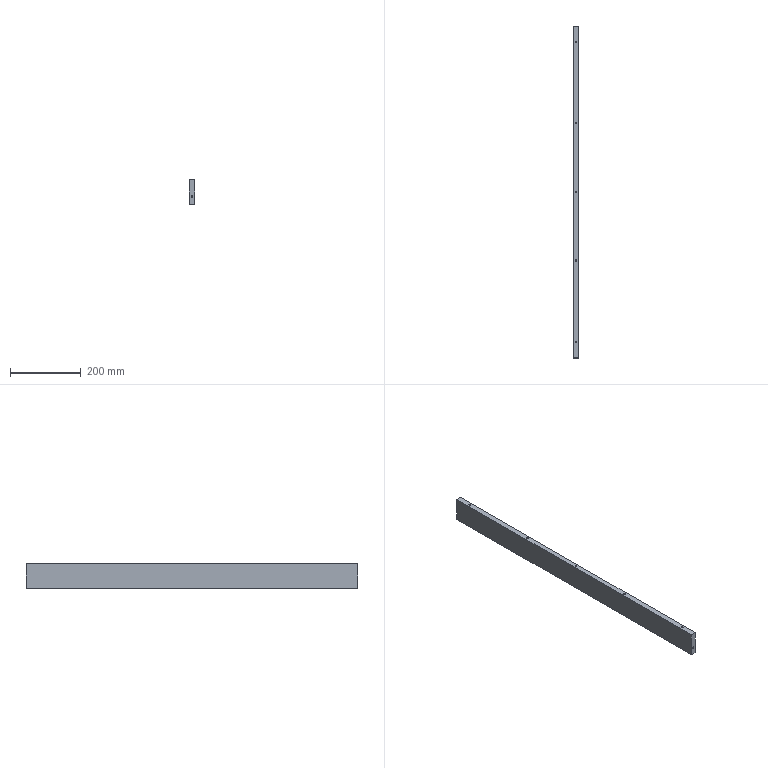Part | STEP file | 0244_206_Rib | 1 solid | 34 faces | box 15 x 940 x 69 mm | volume 970770 mm3 | cylinder 14 | cone 14 | plane 6 | commonest cylinder face diameters 5 x14